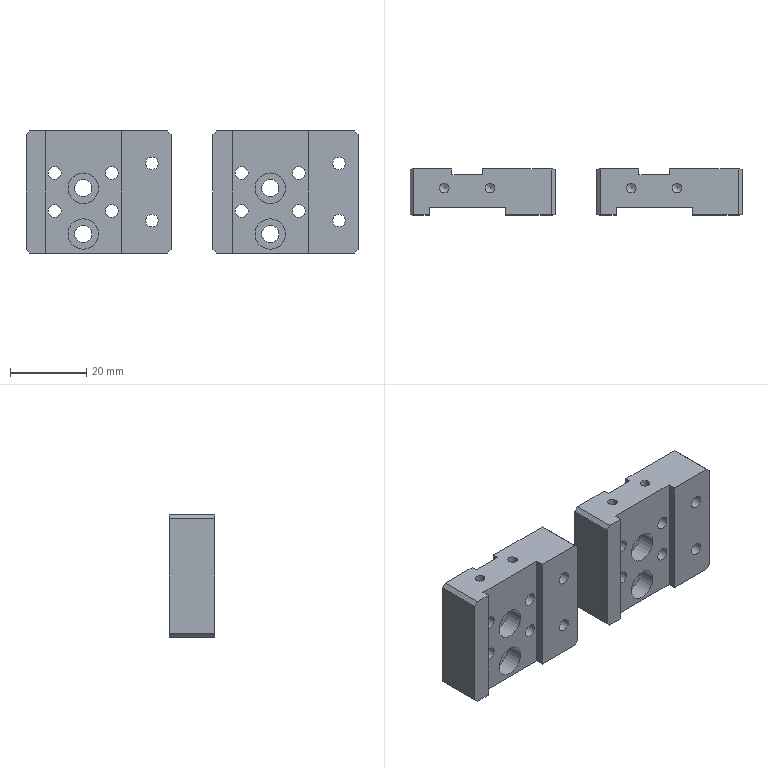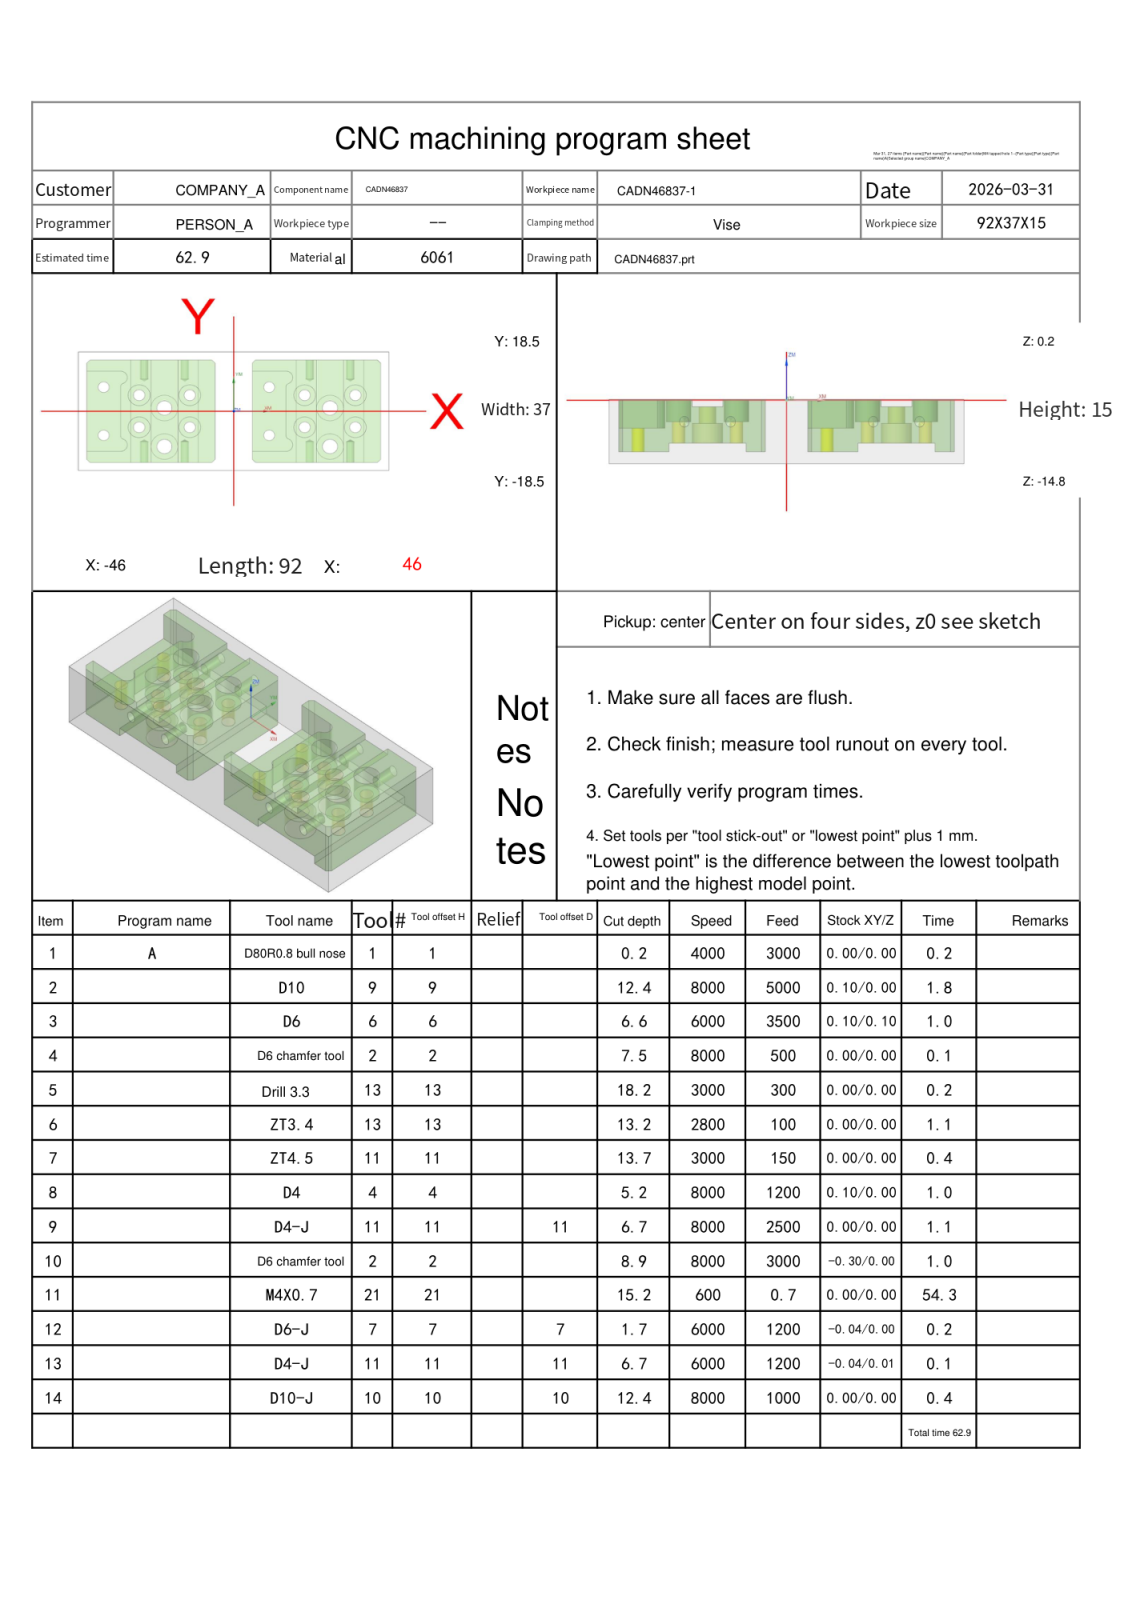NC program | NX | posted by the shop | part box 87 x 12 x 32 mm
Lines 4853 to 5636 of 5636:
N10 T02 M06
(D6 chamfer tool  D=6. R=0. H=02 ce=0.00 di=0.00)
G00 G90 G54 X30.372 Y-.25 M03 S8000
G43 H02 Z20.
M08
Z2.099
G01 Z-1.5 F3000.
G03 X30.672 Y-.33 I.3 J.52
X31.192 Y-.03 I0.0 J.6
G01 X31.2 Y0.0
Y16.
G02 X32.5 Y17.3 I1.3 J0.0
G01 X42.5
X42.754 Y17.275
X42.997 Y17.201
X43.222 Y17.081
X43.419 Y16.919
X44.419 Y15.919
X44.581 Y15.722
X44.701 Y15.497
X44.775 Y15.254
X44.8 Y15.
Y-15.
X44.775 Y-15.254
X44.701 Y-15.497
X44.581 Y-15.722
X44.419 Y-15.919
X43.419 Y-16.919
X43.222 Y-17.081
X42.997 Y-17.201
X42.754 Y-17.275
X42.5 Y-17.3
X32.5
G02 X31.2 Y-16. I0.0 J1.3
G01 Y0.0
X31.192 Y.03
G03 X30.672 Y.33 I-.52 J-.3
X30.372 Y.25 I0.0 J-.6
G01 Z2.099
G00 Z2.25
X26.628
Z2.099
G01 Z-1.5
G03 X26.328 Y.33 I-.3 J-.52
X25.808 Y.03 I0.0 J-.6
G01 X25.8 Y0.0
Y-16.
G02 X24.5 Y-17.3 I-1.3 J0.0
G01 X6.5
X6.246 Y-17.275
X6.003 Y-17.201
X5.778 Y-17.081
X5.581 Y-16.919
X4.581 Y-15.919
X4.419 Y-15.722
X4.299 Y-15.497
X4.225 Y-15.254
X4.2 Y-15.
Y-12.5
G02 X5.5 Y-11.2 I1.3 J0.0
G01 X15.5
G03 X16.2 Y-10.5 I0.0 J.7
X16.074 Y-10.1 I-.7 J0.0
G01 X15.924 Y-9.943
X15.733 Y-9.84
G02 X14.2 Y-7.672 I.767 J2.168
G01 Y7.672
G02 X15.733 Y9.84 I2.3 J0.0
G03 X16.2 Y10.5 I-.233 J.66
X15.908 Y11.069 I-.7 J0.0
G01 X15.714 Y11.166
X15.5 Y11.2
X5.5
G02 X4.2 Y12.5 I0.0 J1.3
G01 Y15.
X4.225 Y15.254
X4.299 Y15.497
X4.419 Y15.722
X4.581 Y15.919
X5.581 Y16.919
X5.778 Y17.081
X6.003 Y17.201
X6.246 Y17.275
X6.5 Y17.3
X24.5
G02 X25.8 Y16. I0.0 J-1.3
G01 Y0.0
X25.808 Y-.03
G03 X26.328 Y-.33 I.52 J.3
X26.628 Y-.25 I0.0 J.6
G01 Z2.099
G00 Z20.
X-18.628
Z2.099
G01 Z-1.5
G03 X-18.328 Y-.33 I.3 J.52
X-17.808 Y-.03 I0.0 J.6
G01 X-17.8 Y0.0
Y16.
G02 X-16.5 Y17.3 I1.3 J0.0
G01 X-6.5
X-6.246 Y17.275
X-6.003 Y17.201
X-5.778 Y17.081
X-5.581 Y16.919
X-4.581 Y15.919
X-4.419 Y15.722
X-4.299 Y15.497
X-4.225 Y15.254
X-4.2 Y15.
Y-15.
X-4.225 Y-15.254
X-4.299 Y-15.497
X-4.419 Y-15.722
X-4.581 Y-15.919
X-5.581 Y-16.919
X-5.778 Y-17.081
X-6.003 Y-17.201
X-6.246 Y-17.275
X-6.5 Y-17.3
X-16.5
G02 X-17.8 Y-16. I0.0 J1.3
G01 Y0.0
X-17.808 Y.03
G03 X-18.328 Y.33 I-.52 J-.3
X-18.628 Y.25 I0.0 J-.6
G01 Z2.099
G00 Z2.25
X-22.372
Z2.099
G01 Z-1.5
G03 X-22.672 Y.33 I-.3 J-.52
X-23.192 Y.03 I0.0 J-.6
G01 X-23.2 Y0.0
Y-16.
G02 X-24.5 Y-17.3 I-1.3 J0.0
G01 X-42.5
X-42.754 Y-17.275
X-42.997 Y-17.201
X-43.222 Y-17.081
X-43.419 Y-16.919
X-44.419 Y-15.919
X-44.581 Y-15.722
X-44.701 Y-15.497
X-44.775 Y-15.254
X-44.8 Y-15.
Y-12.5
G02 X-43.5 Y-11.2 I1.3 J0.0
G01 X-33.5
G03 X-32.8 Y-10.5 I0.0 J.7
X-32.926 Y-10.1 I-.7 J0.0
G01 X-33.076 Y-9.943
X-33.267 Y-9.84
G02 X-34.8 Y-7.672 I.767 J2.168
G01 Y7.672
G02 X-33.267 Y9.84 I2.3 J0.0
G03 X-32.8 Y10.5 I-.233 J.66
X-33.092 Y11.069 I-.7 J0.0
G01 X-33.286 Y11.166
X-33.5 Y11.2
X-43.5
G02 X-44.8 Y12.5 I0.0 J1.3
G01 Y15.
X-44.775 Y15.254
X-44.701 Y15.497
X-44.581 Y15.722
X-44.419 Y15.919
X-43.419 Y16.919
X-43.222 Y17.081
X-42.997 Y17.201
X-42.754 Y17.275
X-42.5 Y17.3
X-24.5
G02 X-23.2 Y16. I0.0 J-1.3
G01 Y0.0
X-23.192 Y-.03
G03 X-22.672 Y-.33 I.52 J.3
X-22.372 Y-.25 I0.0 J.6
G01 Z2.099
G00 Z20.
X-21.813 Y17.3
Z1.755
G01 Z-3.
X-19.188
Z1.755
G00 Z20.
Y-17.3
Z1.755
G01 Z-3.
X-21.813
Z1.755
G00 Z20.
X27.188 Y17.3
Z1.755
G01 Z-3.
X29.813
Z1.755
G00 Z20.
Y-17.3
Z1.755
G01 Z-3.
X27.188
Z1.755
G00 Z20.
X3.455 Y-9.453
Z1.755
G01 Z-8.
G03 X3.725 Y-9.526 I.27 J.468
X4.193 Y-9.256 I0.0 J.54
G01 X4.2 Y-9.229
Y9.229
X4.193 Y9.256
G03 X3.725 Y9.526 I-.468 J-.27
X3.455 Y9.453 I0.0 J-.54
G01 Z1.755
G00 Z20.
X-45.545 Y-9.453
Z1.755
G01 Z-8.
G03 X-45.275 Y-9.526 I.27 J.468
X-44.807 Y-9.256 I0.0 J.54
G01 X-44.8 Y-9.229
Y9.229
X-44.807 Y9.256
G03 X-45.275 Y9.526 I-.468 J-.27
X-45.545 Y9.453 I0.0 J-.54
G01 Z1.755
G00 Z20.
G00 G90 X-38.5 Y-7.5 M03 S8000
Z20.
G98 G81 X-38.5 Y-7.5 Z-8.7 R-3.5 F500.
Y7.5
X10.5
Y-7.5
G80
G00 Z20.
G00 G90 X29.05 Y-10.982 M03 S8000
Z20.
Z-2.
G01 Z-2.5 F500.
X30. Y-10.95
G03 X28.5 Y-9.45 I-1.5 J0.0
X26.95 Y-11. I0.0 J-1.55
X28.5 Y-12.55 I1.55 J0.0
X30.05 Y-11. I0.0 J1.55
X28.5 Y-9.45 I-1.55 J0.0
X27. Y-10.95 I0.0 J-1.5
G01 X27.95 Y-10.982
Z-2.
G00 Z20.
X29.05 Y1.018
Z-2.
G01 Z-2.5
X30. Y1.05
G03 X28.5 Y2.55 I-1.5 J0.0
X26.95 Y1. I0.0 J-1.55
X28.5 Y-.55 I1.55 J0.0
X30.05 Y1. I0.0 J1.55
X28.5 Y2.55 I-1.55 J0.0
X27. Y1.05 I0.0 J-1.5
G01 X27.95 Y1.018
Z-2.
G00 Z20.
X-19.95
Z-2.
G01 Z-2.5
X-19. Y1.05
G03 X-20.5 Y2.55 I-1.5 J0.0
X-22.05 Y1. I0.0 J-1.55
X-20.5 Y-.55 I1.55 J0.0
X-18.95 Y1. I0.0 J1.55
X-20.5 Y2.55 I-1.55 J0.0
X-22. Y1.05 I0.0 J-1.5
G01 X-21.05 Y1.018
Z-2.
G00 Z20.
X-19.95 Y-10.982
Z-2.
G01 Z-2.5
X-19. Y-10.95
G03 X-20.5 Y-9.45 I-1.5 J0.0
X-22.05 Y-11. I0.0 J-1.55
X-20.5 Y-12.55 I1.55 J0.0
X-18.95 Y-11. I0.0 J1.55
X-20.5 Y-9.45 I-1.55 J0.0
X-22. Y-10.95 I0.0 J-1.5
G01 X-21.05 Y-10.982
Z-2.
G00 Z20.
G00 G90 X37.497 Y7.063 M03 S8000
Z20.
Z2.5
G01 X37.44 Y7.108 Z2.474 F500.
X37.147 Y7.281 Z2.35
X36.834 Y7.413 Z2.226
X36.507 Y7.502 Z2.103
X36.17 Y7.547 Z1.979
X35.83 Z1.855
X35.493 Y7.502 Z1.732
X35.166 Y7.413 Z1.608
X34.853 Y7.281 Z1.484
X34.56 Y7.108 Z1.361
X34.293 Y6.898 Z1.237
X34.056 Y6.655 Z1.113
X33.854 Y6.382 Z.99
X33.73 Y6.168 Z.9
X33.595 Y5.856 Z.776
X33.502 Y5.529 Z.652
X33.454 Y5.193 Z.529
X33.451 Y4.853 Z.405
X33.493 Y4.516 Z.281
X33.58 Y4.188 Z.158
X33.709 Y3.873 Z.034
X33.879 Y3.579 Z-.089
X34.086 Y3.31 Z-.213
X34.328 Y3.071 Z-.337
X34.598 Y2.866 Z-.46
X34.894 Y2.699 Z-.584
X35.21 Y2.572 Z-.708
X35.539 Y2.489 Z-.831
X35.876 Y2.45 Z-.955
X36. Z-1.
G03 X38.55 Y5. I0.0 J2.55
X36. Y7.55 I-2.55 J0.0
X33.45 Y5. I0.0 J-2.55
X36. Y2.45 I2.55 J0.0
X36.497 Y2.499 I0.0 J2.55
G01 Z1.5
G00 Z20.
X37.497 Y-2.937
Z2.5
G01 X37.44 Y-2.892 Z2.474
X37.147 Y-2.719 Z2.35
X36.834 Y-2.587 Z2.226
X36.507 Y-2.498 Z2.103
X36.17 Y-2.453 Z1.979
X35.83 Z1.855
X35.493 Y-2.498 Z1.732
X35.166 Y-2.587 Z1.608
X34.853 Y-2.719 Z1.484
X34.56 Y-2.892 Z1.361
X34.293 Y-3.102 Z1.237
X34.056 Y-3.345 Z1.113
X33.854 Y-3.618 Z.99
X33.73 Y-3.832 Z.9
X33.595 Y-4.144 Z.776
X33.502 Y-4.471 Z.652
X33.454 Y-4.807 Z.529
X33.451 Y-5.147 Z.405
X33.493 Y-5.484 Z.281
X33.58 Y-5.812 Z.158
X33.709 Y-6.127 Z.034
X33.879 Y-6.421 Z-.089
X34.086 Y-6.69 Z-.213
X34.328 Y-6.929 Z-.337
X34.598 Y-7.134 Z-.46
X34.894 Y-7.301 Z-.584
X35.21 Y-7.428 Z-.708
X35.539 Y-7.511 Z-.831
X35.876 Y-7.55 Z-.955
X36. Z-1.
G03 X38.55 Y-5. I0.0 J2.55
X36. Y-2.45 I-2.55 J0.0
X33.45 Y-5. I0.0 J-2.55
X36. Y-7.55 I2.55 J0.0
X36.497 Y-7.501 I0.0 J2.55
G01 Z1.5
G00 Z20.
X22.497 Y-2.937
Z2.5
G01 X22.44 Y-2.892 Z2.474
X22.147 Y-2.719 Z2.35
X21.834 Y-2.587 Z2.226
X21.507 Y-2.498 Z2.103
X21.17 Y-2.453 Z1.979
X20.83 Z1.855
X20.493 Y-2.498 Z1.732
X20.166 Y-2.587 Z1.608
X19.853 Y-2.719 Z1.484
X19.56 Y-2.892 Z1.361
X19.293 Y-3.102 Z1.237
X19.056 Y-3.345 Z1.113
X18.854 Y-3.618 Z.99
X18.73 Y-3.832 Z.9
X18.595 Y-4.144 Z.776
X18.502 Y-4.471 Z.652
X18.454 Y-4.807 Z.529
X18.451 Y-5.147 Z.405
X18.493 Y-5.484 Z.281
X18.58 Y-5.812 Z.158
X18.709 Y-6.127 Z.034
X18.879 Y-6.421 Z-.089
X19.086 Y-6.69 Z-.213
X19.328 Y-6.929 Z-.337
X19.598 Y-7.134 Z-.46
X19.894 Y-7.301 Z-.584
X20.21 Y-7.428 Z-.708
X20.539 Y-7.511 Z-.831
X20.876 Y-7.55 Z-.955
X21. Z-1.
G03 X23.55 Y-5. I0.0 J2.55
X21. Y-2.45 I-2.55 J0.0
X18.45 Y-5. I0.0 J-2.55
X21. Y-7.55 I2.55 J0.0
X21.497 Y-7.501 I0.0 J2.55
G01 Z1.5
G00 Z20.
X22.497 Y7.063
Z2.5
G01 X22.44 Y7.108 Z2.474
X22.147 Y7.281 Z2.35
X21.834 Y7.413 Z2.226
X21.507 Y7.502 Z2.103
X21.17 Y7.547 Z1.979
X20.83 Z1.855
X20.493 Y7.502 Z1.732
X20.166 Y7.413 Z1.608
X19.853 Y7.281 Z1.484
X19.56 Y7.108 Z1.361
X19.293 Y6.898 Z1.237
X19.056 Y6.655 Z1.113
X18.854 Y6.382 Z.99
X18.73 Y6.168 Z.9
X18.595 Y5.856 Z.776
X18.502 Y5.529 Z.652
X18.454 Y5.193 Z.529
X18.451 Y4.853 Z.405
X18.493 Y4.516 Z.281
X18.58 Y4.188 Z.158
X18.709 Y3.873 Z.034
X18.879 Y3.579 Z-.089
X19.086 Y3.31 Z-.213
X19.328 Y3.071 Z-.337
X19.598 Y2.866 Z-.46
X19.894 Y2.699 Z-.584
X20.21 Y2.572 Z-.708
X20.539 Y2.489 Z-.831
X20.876 Y2.45 Z-.955
X21. Z-1.
G03 X23.55 Y5. I0.0 J2.55
X21. Y7.55 I-2.55 J0.0
X18.45 Y5. I0.0 J-2.55
X21. Y2.45 I2.55 J0.0
X21.497 Y2.499 I0.0 J2.55
G01 Z1.5
G00 Z20.
X-11.503 Y7.063
Z2.5
G01 X-11.56 Y7.108 Z2.474
X-11.853 Y7.281 Z2.35
X-12.166 Y7.413 Z2.226
X-12.493 Y7.502 Z2.103
X-12.83 Y7.547 Z1.979
X-13.17 Z1.855
X-13.507 Y7.502 Z1.732
X-13.834 Y7.413 Z1.608
X-14.147 Y7.281 Z1.484
X-14.44 Y7.108 Z1.361
X-14.707 Y6.898 Z1.237
X-14.944 Y6.655 Z1.113
X-15.147 Y6.382 Z.99
X-15.27 Y6.168 Z.9
X-15.405 Y5.856 Z.776
X-15.498 Y5.529 Z.652
X-15.546 Y5.193 Z.529
X-15.549 Y4.853 Z.405
X-15.507 Y4.516 Z.281
X-15.42 Y4.188 Z.158
X-15.291 Y3.873 Z.034
X-15.121 Y3.579 Z-.089
X-14.914 Y3.31 Z-.213
X-14.672 Y3.071 Z-.337
X-14.402 Y2.866 Z-.46
X-14.106 Y2.699 Z-.584
X-13.79 Y2.572 Z-.708
X-13.461 Y2.489 Z-.831
X-13.124 Y2.45 Z-.955
X-13. Z-1.
G03 X-10.45 Y5. I0.0 J2.55
X-13. Y7.55 I-2.55 J0.0
X-15.55 Y5. I0.0 J-2.55
X-13. Y2.45 I2.55 J0.0
X-12.503 Y2.499 I0.0 J2.55
G01 Z1.5
G00 Z20.
X-11.503 Y-2.937
Z2.5
G01 X-11.56 Y-2.892 Z2.474
X-11.853 Y-2.719 Z2.35
X-12.166 Y-2.587 Z2.226
X-12.493 Y-2.498 Z2.103
X-12.83 Y-2.453 Z1.979
X-13.17 Z1.855
X-13.507 Y-2.498 Z1.732
X-13.834 Y-2.587 Z1.608
X-14.147 Y-2.719 Z1.484
X-14.44 Y-2.892 Z1.361
X-14.707 Y-3.102 Z1.237
X-14.944 Y-3.345 Z1.113
X-15.147 Y-3.618 Z.99
X-15.27 Y-3.832 Z.9
X-15.405 Y-4.144 Z.776
X-15.498 Y-4.471 Z.652
X-15.546 Y-4.807 Z.529
X-15.549 Y-5.147 Z.405
X-15.507 Y-5.484 Z.281
X-15.42 Y-5.812 Z.158
X-15.291 Y-6.127 Z.034
X-15.121 Y-6.421 Z-.089
X-14.914 Y-6.69 Z-.213
X-14.672 Y-6.929 Z-.337
X-14.402 Y-7.134 Z-.46
X-14.106 Y-7.301 Z-.584
X-13.79 Y-7.428 Z-.708
X-13.461 Y-7.511 Z-.831
X-13.124 Y-7.55 Z-.955
X-13. Z-1.
G03 X-10.45 Y-5. I0.0 J2.55
X-13. Y-2.45 I-2.55 J0.0
X-15.55 Y-5. I0.0 J-2.55
X-13. Y-7.55 I2.55 J0.0
X-12.503 Y-7.501 I0.0 J2.55
G01 Z1.5
G00 Z20.
X-26.503 Y-2.937
Z2.5
G01 X-26.56 Y-2.892 Z2.474
X-26.853 Y-2.719 Z2.35
X-27.166 Y-2.587 Z2.226
X-27.493 Y-2.498 Z2.103
X-27.83 Y-2.453 Z1.979
X-28.17 Z1.855
X-28.507 Y-2.498 Z1.732
X-28.834 Y-2.587 Z1.608
X-29.147 Y-2.719 Z1.484
X-29.44 Y-2.892 Z1.361
X-29.707 Y-3.102 Z1.237
X-29.944 Y-3.345 Z1.113
X-30.147 Y-3.618 Z.99
X-30.27 Y-3.832 Z.9
X-30.405 Y-4.144 Z.776
X-30.498 Y-4.471 Z.652
X-30.546 Y-4.807 Z.529
X-30.549 Y-5.147 Z.405
X-30.507 Y-5.484 Z.281
X-30.42 Y-5.812 Z.158
X-30.291 Y-6.127 Z.034
X-30.121 Y-6.421 Z-.089
X-29.914 Y-6.69 Z-.213
X-29.672 Y-6.929 Z-.337
X-29.402 Y-7.134 Z-.46
X-29.106 Y-7.301 Z-.584
X-28.79 Y-7.428 Z-.708
X-28.461 Y-7.511 Z-.831
X-28.124 Y-7.55 Z-.955
X-28. Z-1.
G03 X-25.45 Y-5. I0.0 J2.55
X-28. Y-2.45 I-2.55 J0.0
X-30.55 Y-5. I0.0 J-2.55
X-28. Y-7.55 I2.55 J0.0
X-27.503 Y-7.501 I0.0 J2.55
G01 Z1.5
G00 Z20.
X-26.503 Y7.063
Z2.5
G01 X-26.56 Y7.108 Z2.474
X-26.853 Y7.281 Z2.35
X-27.166 Y7.413 Z2.226
X-27.493 Y7.502 Z2.103
X-27.83 Y7.547 Z1.979
X-28.17 Z1.855
X-28.507 Y7.502 Z1.732
X-28.834 Y7.413 Z1.608
X-29.147 Y7.281 Z1.484
X-29.44 Y7.108 Z1.361
X-29.707 Y6.898 Z1.237
X-29.944 Y6.655 Z1.113
X-30.147 Y6.382 Z.99
X-30.27 Y6.168 Z.9
X-30.405 Y5.856 Z.776
X-30.498 Y5.529 Z.652
X-30.546 Y5.193 Z.529
X-30.549 Y4.853 Z.405
X-30.507 Y4.516 Z.281
X-30.42 Y4.188 Z.158
X-30.291 Y3.873 Z.034
X-30.121 Y3.579 Z-.089
X-29.914 Y3.31 Z-.213
X-29.672 Y3.071 Z-.337
X-29.402 Y2.866 Z-.46
X-29.106 Y2.699 Z-.584
X-28.79 Y2.572 Z-.708
X-28.461 Y2.489 Z-.831
X-28.124 Y2.45 Z-.955
X-28. Z-1.
G03 X-25.45 Y5. I0.0 J2.55
X-28. Y7.55 I-2.55 J0.0
X-30.55 Y5. I0.0 J-2.55
X-28. Y2.45 I2.55 J0.0
X-27.503 Y2.499 I0.0 J2.55
G01 Z1.5
G00 Z20.
G91 G28 Z0.0
M05
M09
G91 G28 Z0.0
M01
N11 T21 M06
(M4X0.7 D=3.3 DR_a=180 H=21)
G00 G90 G54 X-38.5 Y-7.5 M03 S600
G43 H21 Z20.
M08
G95
G98 G84 X-38.5 Y-7.5 Z-15. R-5.5 F.7 Q4.
Y7.5
X10.5
Y-7.5
G80
G94
G00 Z20.
G91 G28 Z0.0
M05
M09
G91 G28 Z0.0
M01
N12 T07 M06
(D6-J  D=6. R=0. H=07 ce=-0.04 di=0.00)
G00 G90 G54 X28.565 Y19.7 M03 S6000
G43 H07 Z20.
M08
Z-1.
G01 Z-1.5 F1200.
G41 D07
X28.465
G03 X27.465 Y18.7 I0.0 J-1.
G01 Y-18.7
G03 X28.465 Y-19.7 I1. J0.0
G01 G40 X28.565
X28.435
G41 D07
X28.535
G03 X29.535 Y-18.7 I0.0 J1.
G01 Y18.7
G03 X28.535 Y19.7 I-1. J0.0
G01 G40 X28.435
Z-1.
G00 Z20.
X-20.435
Z-1.
G01 Z-1.5
G41 D07
X-20.535
G03 X-21.535 Y18.7 I0.0 J-1.
G01 Y-18.7
G03 X-20.535 Y-19.7 I1. J0.0
G01 G40 X-20.435
X-20.565
G41 D07
X-20.465
G03 X-19.465 Y-18.7 I0.0 J1.
G01 Y18.7
G03 X-20.465 Y19.7 I-1. J0.0
G01 G40 X-20.565
Z-1.
G00 Z20.
G91 G28 Z0.0
M05
M09
G91 G28 Z0.0
M01
N13 T11 M06
(D4-J  D=4. R=0. H=11 ce=-0.04 di=0.01)
G00 G90 G54 X2.7 Y-9.435 M03 S6000
G43 H11 Z20.
M08
Z-5.995
G01 Z-6.495 F1200.
G41 D11
Y-9.535
G03 X3.7 Y-10.535 I1. J0.0
G01 X15.5
X15.536 Y-10.527
X15.543 Y-10.487
X15.512 Y-10.467
G02 X13.535 Y-7.672 I.988 J2.795
G01 Y7.672
G02 X15.512 Y10.467 I2.965 J0.0
G01 X15.543 Y10.487
X15.536 Y10.527
X15.5 Y10.535
X3.7
G03 X2.7 Y9.535 I0.0 J-1.
G01 G40 Y9.435
Z-5.995
G00 Z20.
X-46.3 Y-9.435
Z-5.995
G01 Z-6.495
G41 D11
Y-9.535
G03 X-45.3 Y-10.535 I1. J0.0
G01 X-33.5
X-33.464 Y-10.527
X-33.457 Y-10.487
X-33.488 Y-10.467
G02 X-35.465 Y-7.672 I.988 J2.795
G01 Y7.672
G02 X-33.488 Y10.467 I2.965 J0.0
G01 X-33.457 Y10.487
X-33.464 Y10.527
X-33.5 Y10.535
X-45.3
G03 X-46.3 Y9.535 I0.0 J-1.
G01 G40 Y9.435
Z-5.995
G00 Z20.
G91 G28 Z0.0
M05
M09
G91 G28 Z0.0
M01
N14 T10 M06
(D10-J  D=10. R=0. H=10 ce=0.00 di=0.00)
G00 G90 G54 X5.487 Y22.116 M03 S8000
G43 H10 Z20.
M08
Z-11.7
G01 Z-12.2 F1000.
G41 D10
X5.503 Y21.917
G03 X6.5 Y21. I.997 J.083
G01 X42.5
G02 X46.036 Y19.536 I0.0 J-5.
G01 X47.036 Y18.536
G02 X48.5 Y15. I-3.536 J-3.536
G01 Y-15.
G02 X47.036 Y-18.536 I-5. J0.0
G01 X46.036 Y-19.536
G02 X42.5 Y-21. I-3.536 J3.536
G01 X6.5
G02 X2.964 Y-19.536 I0.0 J5.
G01 X1.964 Y-18.536
G02 X.5 Y-15. I3.536 J3.536
G01 Y15.
G02 X1.964 Y18.536 I5. J0.0
G01 X2.964 Y19.536
G02 X6.5 Y21. I3.536 J-3.536
G01 X7.
G03 X8. Y22. I0.0 J1.
G01 G40 Y22.2
X-.483 Y18.641
G41 D10
X-.654 Y18.537
G03 X-1.133 Y17.683 I.52 J-.854
X-1.028 Y17.236 I1. J0.0
G02 X-.5 Y15. I-4.472 J-2.236
G01 Y-15.
G02 X-1.964 Y-18.536 I-5. J0.0
G01 X-2.964 Y-19.536
G02 X-6.5 Y-21. I-3.536 J3.536
G01 X-42.5
G02 X-46.036 Y-19.536 I0.0 J5.
G01 X-47.036 Y-18.536
G02 X-48.5 Y-15. I3.536 J3.536
G01 Y15.
G02 X-47.036 Y18.536 I5. J0.0
G01 X-46.036 Y19.536
G02 X-42.5 Y21. I3.536 J-3.536
G01 X-6.5
G02 X-2.964 Y19.536 I0.0 J-5.
G01 X-1.964 Y18.536
G02 X-1.028 Y17.236 I-3.536 J-3.536
X-.827 Y16.778 I-4.472 J-2.236
G03 X.108 Y16.134 I.935 J.356
X.463 Y16.2 I0.0 J1.
G01 G40 X0.0 Y17.398
Z-11.7
G00 Z20.
M05
M09
G91 G28 Z0.0
G91 G28 Y0.0
M30
%